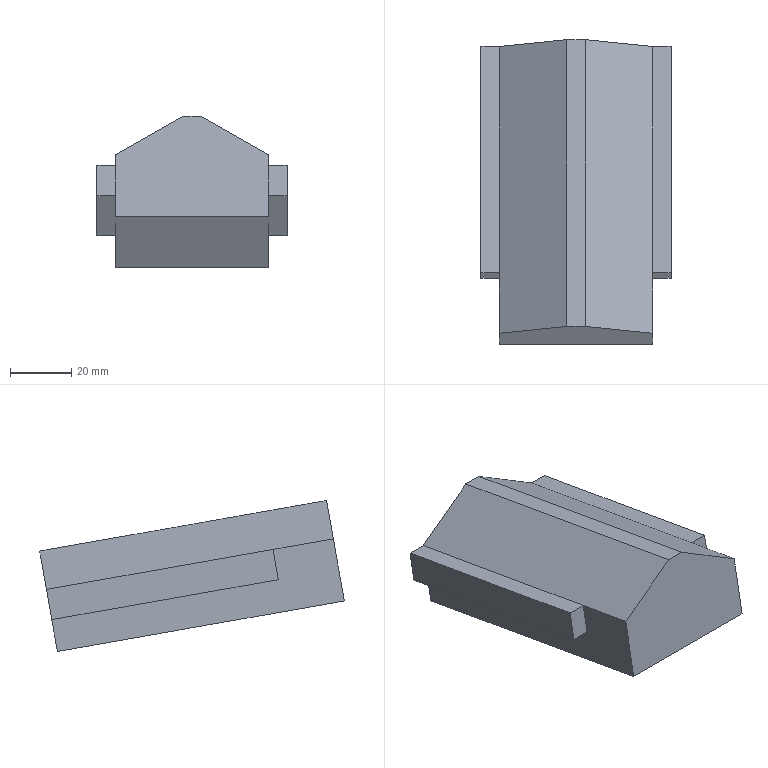Part | NX | features solid 2 | 1 solid | 16 faces | box 62 x 99.334 x 49.259 mm | volume 140476 mm3 | plane 16
STEP:
#1=CARTESIAN_POINT('',(-435.,-638.798,-53.975));
#2=VERTEX_POINT('',#1);
#3=CARTESIAN_POINT('',(-435.,-640.633,-64.38));
#4=VERTEX_POINT('',#3);
#5=CARTESIAN_POINT('',(-435.,-637.061,-44.126));
#6=DIRECTION('',(0.,-0.1736,-0.9848));
#7=VECTOR('',#6,1000.);
#8=LINE('',#5,#7);
#9=EDGE_CURVE('',#2,#4,#8,.T.);
#10=ORIENTED_EDGE('',*,*,#9,.T.);
#11=CARTESIAN_POINT('',(-435.,-734.189,-47.884));
#12=VERTEX_POINT('',#11);
#13=CARTESIAN_POINT('',(-435.,-734.189,-47.884));
#14=DIRECTION('',(0.,0.9848,-0.1736));
#15=VECTOR('',#14,1000.);
#16=LINE('',#13,#15);
#17=EDGE_CURVE('',#12,#4,#16,.T.);
#18=ORIENTED_EDGE('',*,*,#17,.F.);
#19=CARTESIAN_POINT('',(-435.,-732.354,-37.478));
#20=VERTEX_POINT('',#19);
#21=CARTESIAN_POINT('',(-435.,-730.618,-27.63));
#22=DIRECTION('',(0.,-0.1736,-0.9848));
#23=VECTOR('',#22,1000.);
#24=LINE('',#21,#23);
#25=EDGE_CURVE('',#20,#12,#24,.T.);
#26=ORIENTED_EDGE('',*,*,#25,.F.);
#27=CARTESIAN_POINT('',(-435.,-730.618,-27.63));
#28=VERTEX_POINT('',#27);
#29=CARTESIAN_POINT('',(-435.,-730.618,-27.63));
#30=CARTESIAN_POINT('',(-435.,-731.197,-30.913));
#31=CARTESIAN_POINT('',(-435.,-731.776,-34.195));
#32=CARTESIAN_POINT('',(-435.,-732.354,-37.478));
#33=B_SPLINE_CURVE_WITH_KNOTS('',3,(#29,#30,#31,#32),.UNSPECIFIED.,.F.,.F.,(4,4),(0.,1.),.PIECEWISE_BEZIER_KNOTS.);
#34=EDGE_CURVE('',#28,#20,#33,.T.);
#35=ORIENTED_EDGE('',*,*,#34,.F.);
#36=CARTESIAN_POINT('',(-435.,-710.922,-31.103));
#37=VERTEX_POINT('',#36);
#38=CARTESIAN_POINT('',(-435.,-710.922,-31.103));
#39=CARTESIAN_POINT('',(-435.,-717.487,-29.945));
#40=CARTESIAN_POINT('',(-435.,-724.053,-28.788));
#41=CARTESIAN_POINT('',(-435.,-730.618,-27.63));
#42=B_SPLINE_CURVE_WITH_KNOTS('',3,(#38,#39,#40,#41),.UNSPECIFIED.,.F.,.F.,(4,4),(0.,1.),.UNSPECIFIED.);
#43=EDGE_CURVE('',#28,#37,#42,.F.);
#44=ORIENTED_EDGE('',*,*,#43,.T.);
#45=CARTESIAN_POINT('',(-435.,-712.658,-40.951));
#46=VERTEX_POINT('',#45);
#47=CARTESIAN_POINT('',(-435.,-710.922,-31.103));
#48=CARTESIAN_POINT('',(-435.,-711.501,-34.386));
#49=CARTESIAN_POINT('',(-435.,-712.079,-37.668));
#50=CARTESIAN_POINT('',(-435.,-712.658,-40.951));
#51=B_SPLINE_CURVE_WITH_KNOTS('',3,(#47,#48,#49,#50),.UNSPECIFIED.,.F.,.F.,(4,4),(0.,1.),.PIECEWISE_BEZIER_KNOTS.);
#52=EDGE_CURVE('',#37,#46,#51,.T.);
#53=ORIENTED_EDGE('',*,*,#52,.T.);
#54=CARTESIAN_POINT('',(-435.,-673.266,-47.897));
#55=VERTEX_POINT('',#54);
#56=CARTESIAN_POINT('',(-435.,-732.354,-37.478));
#57=CARTESIAN_POINT('',(-435.,-712.658,-40.951));
#58=CARTESIAN_POINT('',(-435.,-692.962,-44.424));
#59=CARTESIAN_POINT('',(-435.,-673.266,-47.897));
#60=B_SPLINE_CURVE_WITH_KNOTS('',3,(#56,#57,#58,#59),.UNSPECIFIED.,.F.,.F.,(4,4),(0.,1.),.PIECEWISE_BEZIER_KNOTS.);
#61=EDGE_CURVE('',#55,#46,#60,.F.);
#62=ORIENTED_EDGE('',*,*,#61,.F.);
#63=CARTESIAN_POINT('',(-435.,-638.798,-53.975));
#64=DIRECTION('',(0.,-0.9848,0.1736));
#65=VECTOR('',#64,1000.);
#66=LINE('',#63,#65);
#67=EDGE_CURVE('',#2,#55,#66,.T.);
#68=ORIENTED_EDGE('',*,*,#67,.F.);
#69=EDGE_LOOP('',(#10,#18,#26,#35,#44,#53,#62,#68));
#70=FACE_BOUND('',#69,.T.);
#71=CARTESIAN_POINT('',(-435.,-730.618,-27.63));
#72=DIRECTION('',(-1.,0.,0.));
#73=DIRECTION('',(0.,0.342,-0.9397));
#74=AXIS2_PLACEMENT_3D('',#71,#72,#73);
#75=PLANE('',#74);
#76=ADVANCED_FACE('',(#70),#75,.T.);
#77=CARTESIAN_POINT('',(-385.,-730.618,-27.63));
#78=VERTEX_POINT('',#77);
#79=CARTESIAN_POINT('',(-385.,-732.354,-37.478));
#80=VERTEX_POINT('',#79);
#81=CARTESIAN_POINT('',(-385.,-730.618,-27.63));
#82=CARTESIAN_POINT('',(-385.,-731.197,-30.913));
#83=CARTESIAN_POINT('',(-385.,-731.776,-34.195));
#84=CARTESIAN_POINT('',(-385.,-732.354,-37.478));
#85=B_SPLINE_CURVE_WITH_KNOTS('',3,(#81,#82,#83,#84),.UNSPECIFIED.,.F.,.F.,(4,4),(0.,1.),.PIECEWISE_BEZIER_KNOTS.);
#86=EDGE_CURVE('',#78,#80,#85,.T.);
#87=ORIENTED_EDGE('',*,*,#86,.F.);
#88=CARTESIAN_POINT('',(-407.,-728.412,-15.121));
#89=VERTEX_POINT('',#88);
#90=CARTESIAN_POINT('',(-407.,-728.412,-15.121));
#91=DIRECTION('',(0.866,-0.08682,-0.4924));
#92=VECTOR('',#91,1000.);
#93=LINE('',#90,#92);
#94=EDGE_CURVE('',#89,#78,#93,.T.);
#95=ORIENTED_EDGE('',*,*,#94,.F.);
#96=CARTESIAN_POINT('',(-413.,-728.412,-15.121));
#97=VERTEX_POINT('',#96);
#98=CARTESIAN_POINT('',(-413.,-728.412,-15.121));
#99=DIRECTION('',(1.,0.,0.));
#100=VECTOR('',#99,1000.);
#101=LINE('',#98,#100);
#102=EDGE_CURVE('',#97,#89,#101,.T.);
#103=ORIENTED_EDGE('',*,*,#102,.F.);
#104=CARTESIAN_POINT('',(-435.,-730.618,-27.63));
#105=DIRECTION('',(0.866,0.08682,0.4924));
#106=VECTOR('',#105,1000.);
#107=LINE('',#104,#106);
#108=EDGE_CURVE('',#28,#97,#107,.T.);
#109=ORIENTED_EDGE('',*,*,#108,.F.);
#110=ORIENTED_EDGE('',*,*,#34,.T.);
#111=ORIENTED_EDGE('',*,*,#25,.T.);
#112=CARTESIAN_POINT('',(-385.,-734.189,-47.884));
#113=VERTEX_POINT('',#112);
#114=CARTESIAN_POINT('',(-435.,-734.189,-47.884));
#115=DIRECTION('',(1.,0.,0.));
#116=VECTOR('',#115,1000.);
#117=LINE('',#114,#116);
#118=EDGE_CURVE('',#12,#113,#117,.T.);
#119=ORIENTED_EDGE('',*,*,#118,.T.);
#120=CARTESIAN_POINT('',(-385.,-730.618,-27.63));
#121=DIRECTION('',(0.,-0.1736,-0.9848));
#122=VECTOR('',#121,1000.);
#123=LINE('',#120,#122);
#124=EDGE_CURVE('',#80,#113,#123,.T.);
#125=ORIENTED_EDGE('',*,*,#124,.F.);
#126=EDGE_LOOP('',(#87,#95,#103,#109,#110,#111,#119,#125));
#127=FACE_BOUND('',#126,.T.);
#128=CARTESIAN_POINT('',(-385.,-734.189,-47.884));
#129=DIRECTION('',(0.,-0.9848,0.1736));
#130=DIRECTION('',(0.,-0.1736,-0.9848));
#131=AXIS2_PLACEMENT_3D('',#128,#129,#130);
#132=PLANE('',#131);
#133=ADVANCED_FACE('',(#127),#132,.T.);
#134=CARTESIAN_POINT('',(-385.,-640.633,-64.38));
#135=VERTEX_POINT('',#134);
#136=CARTESIAN_POINT('',(-435.,-640.633,-64.38));
#137=DIRECTION('',(1.,0.,0.));
#138=VECTOR('',#137,1000.);
#139=LINE('',#136,#138);
#140=EDGE_CURVE('',#4,#135,#139,.T.);
#141=ORIENTED_EDGE('',*,*,#140,.T.);
#142=CARTESIAN_POINT('',(-385.,-734.189,-47.884));
#143=DIRECTION('',(0.,0.9848,-0.1736));
#144=VECTOR('',#143,1000.);
#145=LINE('',#142,#144);
#146=EDGE_CURVE('',#113,#135,#145,.T.);
#147=ORIENTED_EDGE('',*,*,#146,.F.);
#148=ORIENTED_EDGE('',*,*,#118,.F.);
#149=ORIENTED_EDGE('',*,*,#17,.T.);
#150=EDGE_LOOP('',(#141,#147,#148,#149));
#151=FACE_BOUND('',#150,.T.);
#152=CARTESIAN_POINT('',(-435.,-734.189,-47.884));
#153=DIRECTION('',(0.,-0.1736,-0.9848));
#154=DIRECTION('',(0.,0.9848,-0.1736));
#155=AXIS2_PLACEMENT_3D('',#152,#153,#154);
#156=PLANE('',#155);
#157=ADVANCED_FACE('',(#151),#156,.T.);
#158=CARTESIAN_POINT('',(-385.,-712.658,-40.951));
#159=VERTEX_POINT('',#158);
#160=CARTESIAN_POINT('',(-385.,-673.266,-47.897));
#161=VERTEX_POINT('',#160);
#162=CARTESIAN_POINT('',(-385.,-732.354,-37.478));
#163=CARTESIAN_POINT('',(-385.,-712.658,-40.951));
#164=CARTESIAN_POINT('',(-385.,-692.962,-44.424));
#165=CARTESIAN_POINT('',(-385.,-673.266,-47.897));
#166=B_SPLINE_CURVE_WITH_KNOTS('',3,(#162,#163,#164,#165),.UNSPECIFIED.,.F.,.F.,(4,4),(0.,1.),.PIECEWISE_BEZIER_KNOTS.);
#167=EDGE_CURVE('',#159,#161,#166,.T.);
#168=ORIENTED_EDGE('',*,*,#167,.F.);
#169=CARTESIAN_POINT('',(-385.,-710.922,-31.103));
#170=VERTEX_POINT('',#169);
#171=CARTESIAN_POINT('',(-385.,-710.922,-31.103));
#172=CARTESIAN_POINT('',(-385.,-711.501,-34.386));
#173=CARTESIAN_POINT('',(-385.,-712.079,-37.668));
#174=CARTESIAN_POINT('',(-385.,-712.658,-40.951));
#175=B_SPLINE_CURVE_WITH_KNOTS('',3,(#171,#172,#173,#174),.UNSPECIFIED.,.F.,.F.,(4,4),(0.,1.),.PIECEWISE_BEZIER_KNOTS.);
#176=EDGE_CURVE('',#170,#159,#175,.T.);
#177=ORIENTED_EDGE('',*,*,#176,.F.);
#178=CARTESIAN_POINT('',(-385.,-730.618,-27.63));
#179=CARTESIAN_POINT('',(-385.,-724.053,-28.788));
#180=CARTESIAN_POINT('',(-385.,-717.487,-29.945));
#181=CARTESIAN_POINT('',(-385.,-710.922,-31.103));
#182=B_SPLINE_CURVE_WITH_KNOTS('',3,(#178,#179,#180,#181),.UNSPECIFIED.,.F.,.F.,(4,4),(0.,1.),.UNSPECIFIED.);
#183=EDGE_CURVE('',#78,#170,#182,.T.);
#184=ORIENTED_EDGE('',*,*,#183,.F.);
#185=ORIENTED_EDGE('',*,*,#86,.T.);
#186=ORIENTED_EDGE('',*,*,#124,.T.);
#187=ORIENTED_EDGE('',*,*,#146,.T.);
#188=CARTESIAN_POINT('',(-385.,-638.798,-53.975));
#189=VERTEX_POINT('',#188);
#190=CARTESIAN_POINT('',(-385.,-637.061,-44.126));
#191=DIRECTION('',(0.,-0.1736,-0.9848));
#192=VECTOR('',#191,1000.);
#193=LINE('',#190,#192);
#194=EDGE_CURVE('',#189,#135,#193,.T.);
#195=ORIENTED_EDGE('',*,*,#194,.F.);
#196=CARTESIAN_POINT('',(-385.,-638.798,-53.975));
#197=DIRECTION('',(0.,-0.9848,0.1736));
#198=VECTOR('',#197,1000.);
#199=LINE('',#196,#198);
#200=EDGE_CURVE('',#161,#189,#199,.F.);
#201=ORIENTED_EDGE('',*,*,#200,.F.);
#202=EDGE_LOOP('',(#168,#177,#184,#185,#186,#187,#195,#201));
#203=FACE_BOUND('',#202,.T.);
#204=CARTESIAN_POINT('',(-385.,-730.618,-27.63));
#205=DIRECTION('',(-1.,0.,0.));
#206=DIRECTION('',(0.,0.9397,0.342));
#207=AXIS2_PLACEMENT_3D('',#204,#205,#206);
#208=PLANE('',#207);
#209=ADVANCED_FACE('',(#203),#208,.F.);
#210=CARTESIAN_POINT('',(-407.,-634.856,-31.618));
#211=VERTEX_POINT('',#210);
#212=CARTESIAN_POINT('',(-385.,-637.061,-44.126));
#213=VERTEX_POINT('',#212);
#214=CARTESIAN_POINT('',(-407.,-634.856,-31.618));
#215=DIRECTION('',(0.866,-0.08682,-0.4924));
#216=VECTOR('',#215,1000.);
#217=LINE('',#214,#216);
#218=EDGE_CURVE('',#211,#213,#217,.T.);
#219=ORIENTED_EDGE('',*,*,#218,.F.);
#220=CARTESIAN_POINT('',(-407.,-728.412,-15.121));
#221=DIRECTION('',(0.,0.9848,-0.1736));
#222=VECTOR('',#221,1000.);
#223=LINE('',#220,#222);
#224=EDGE_CURVE('',#89,#211,#223,.T.);
#225=ORIENTED_EDGE('',*,*,#224,.F.);
#226=ORIENTED_EDGE('',*,*,#94,.T.);
#227=ORIENTED_EDGE('',*,*,#183,.T.);
#228=CARTESIAN_POINT('',(-385.,-671.53,-38.049));
#229=VERTEX_POINT('',#228);
#230=CARTESIAN_POINT('',(-385.,-730.618,-27.63));
#231=DIRECTION('',(0.,0.9848,-0.1736));
#232=VECTOR('',#231,1000.);
#233=LINE('',#230,#232);
#234=EDGE_CURVE('',#170,#229,#233,.T.);
#235=ORIENTED_EDGE('',*,*,#234,.T.);
#236=CARTESIAN_POINT('',(-385.,-637.061,-44.126));
#237=CARTESIAN_POINT('',(-385.,-648.551,-42.101));
#238=CARTESIAN_POINT('',(-385.,-660.04,-40.075));
#239=CARTESIAN_POINT('',(-385.,-671.53,-38.049));
#240=B_SPLINE_CURVE_WITH_KNOTS('',3,(#236,#237,#238,#239),.UNSPECIFIED.,.F.,.F.,(4,4),(0.,1.),.UNSPECIFIED.);
#241=EDGE_CURVE('',#229,#213,#240,.F.);
#242=ORIENTED_EDGE('',*,*,#241,.T.);
#243=EDGE_LOOP('',(#219,#225,#226,#227,#235,#242));
#244=FACE_BOUND('',#243,.T.);
#245=CARTESIAN_POINT('',(-407.,-728.412,-15.121));
#246=DIRECTION('',(-0.5,-0.1504,-0.8529));
#247=DIRECTION('',(0.8321,0.1897,-0.5212));
#248=AXIS2_PLACEMENT_3D('',#245,#246,#247);
#249=PLANE('',#248);
#250=ADVANCED_FACE('',(#244),#249,.F.);
#251=CARTESIAN_POINT('',(-413.,-634.856,-31.618));
#252=VERTEX_POINT('',#251);
#253=CARTESIAN_POINT('',(-413.,-634.856,-31.618));
#254=DIRECTION('',(1.,0.,0.));
#255=VECTOR('',#254,1000.);
#256=LINE('',#253,#255);
#257=EDGE_CURVE('',#252,#211,#256,.T.);
#258=ORIENTED_EDGE('',*,*,#257,.F.);
#259=CARTESIAN_POINT('',(-413.,-728.412,-15.121));
#260=DIRECTION('',(0.,0.9848,-0.1736));
#261=VECTOR('',#260,1000.);
#262=LINE('',#259,#261);
#263=EDGE_CURVE('',#97,#252,#262,.T.);
#264=ORIENTED_EDGE('',*,*,#263,.F.);
#265=ORIENTED_EDGE('',*,*,#102,.T.);
#266=ORIENTED_EDGE('',*,*,#224,.T.);
#267=EDGE_LOOP('',(#258,#264,#265,#266));
#268=FACE_BOUND('',#267,.T.);
#269=CARTESIAN_POINT('',(-413.,-728.412,-15.121));
#270=DIRECTION('',(0.,-0.1736,-0.9848));
#271=DIRECTION('',(0.,0.9848,-0.1736));
#272=AXIS2_PLACEMENT_3D('',#269,#270,#271);
#273=PLANE('',#272);
#274=ADVANCED_FACE('',(#268),#273,.F.);
#275=CARTESIAN_POINT('',(-435.,-637.061,-44.126));
#276=VERTEX_POINT('',#275);
#277=CARTESIAN_POINT('',(-435.,-637.061,-44.126));
#278=DIRECTION('',(0.866,0.08682,0.4924));
#279=VECTOR('',#278,1000.);
#280=LINE('',#277,#279);
#281=EDGE_CURVE('',#276,#252,#280,.T.);
#282=ORIENTED_EDGE('',*,*,#281,.F.);
#283=CARTESIAN_POINT('',(-435.,-671.53,-38.049));
#284=VERTEX_POINT('',#283);
#285=CARTESIAN_POINT('',(-435.,-671.53,-38.049));
#286=CARTESIAN_POINT('',(-435.,-660.04,-40.075));
#287=CARTESIAN_POINT('',(-435.,-648.551,-42.101));
#288=CARTESIAN_POINT('',(-435.,-637.061,-44.126));
#289=B_SPLINE_CURVE_WITH_KNOTS('',3,(#285,#286,#287,#288),.UNSPECIFIED.,.F.,.F.,(4,4),(0.,1.),.UNSPECIFIED.);
#290=EDGE_CURVE('',#284,#276,#289,.T.);
#291=ORIENTED_EDGE('',*,*,#290,.F.);
#292=CARTESIAN_POINT('',(-435.,-730.618,-27.63));
#293=DIRECTION('',(0.,0.9848,-0.1736));
#294=VECTOR('',#293,1000.);
#295=LINE('',#292,#294);
#296=EDGE_CURVE('',#37,#284,#295,.T.);
#297=ORIENTED_EDGE('',*,*,#296,.F.);
#298=ORIENTED_EDGE('',*,*,#43,.F.);
#299=ORIENTED_EDGE('',*,*,#108,.T.);
#300=ORIENTED_EDGE('',*,*,#263,.T.);
#301=EDGE_LOOP('',(#282,#291,#297,#298,#299,#300));
#302=FACE_BOUND('',#301,.T.);
#303=CARTESIAN_POINT('',(-435.,-730.618,-27.63));
#304=DIRECTION('',(0.5,-0.1504,-0.8529));
#305=DIRECTION('',(0.8321,-0.1897,0.5212));
#306=AXIS2_PLACEMENT_3D('',#303,#304,#305);
#307=PLANE('',#306);
#308=ADVANCED_FACE('',(#302),#307,.F.);
#309=ORIENTED_EDGE('',*,*,#140,.F.);
#310=ORIENTED_EDGE('',*,*,#9,.F.);
#311=CARTESIAN_POINT('',(-441.,-638.798,-53.975));
#312=VERTEX_POINT('',#311);
#313=CARTESIAN_POINT('',(-441.,-638.798,-53.975));
#314=DIRECTION('',(1.,0.,0.));
#315=VECTOR('',#314,1000.);
#316=LINE('',#313,#315);
#317=EDGE_CURVE('',#312,#2,#316,.T.);
#318=ORIENTED_EDGE('',*,*,#317,.F.);
#319=CARTESIAN_POINT('',(-441.,-637.061,-44.126));
#320=VERTEX_POINT('',#319);
#321=CARTESIAN_POINT('',(-441.,-637.061,-44.126));
#322=CARTESIAN_POINT('',(-441.,-637.64,-47.409));
#323=CARTESIAN_POINT('',(-441.,-638.219,-50.692));
#324=CARTESIAN_POINT('',(-441.,-638.798,-53.975));
#325=B_SPLINE_CURVE_WITH_KNOTS('',3,(#321,#322,#323,#324),.UNSPECIFIED.,.F.,.F.,(4,4),(0.,1.),.PIECEWISE_BEZIER_KNOTS.);
#326=EDGE_CURVE('',#320,#312,#325,.T.);
#327=ORIENTED_EDGE('',*,*,#326,.F.);
#328=CARTESIAN_POINT('',(-441.,-637.061,-44.126));
#329=DIRECTION('',(1.,0.,0.));
#330=VECTOR('',#329,1000.);
#331=LINE('',#328,#330);
#332=EDGE_CURVE('',#320,#276,#331,.T.);
#333=ORIENTED_EDGE('',*,*,#332,.T.);
#334=ORIENTED_EDGE('',*,*,#281,.T.);
#335=ORIENTED_EDGE('',*,*,#257,.T.);
#336=ORIENTED_EDGE('',*,*,#218,.T.);
#337=CARTESIAN_POINT('',(-379.,-637.061,-44.126));
#338=VERTEX_POINT('',#337);
#339=CARTESIAN_POINT('',(-379.,-637.061,-44.126));
#340=DIRECTION('',(-1.,0.,0.));
#341=VECTOR('',#340,1000.);
#342=LINE('',#339,#341);
#343=EDGE_CURVE('',#338,#213,#342,.T.);
#344=ORIENTED_EDGE('',*,*,#343,.F.);
#345=CARTESIAN_POINT('',(-379.,-638.798,-53.975));
#346=VERTEX_POINT('',#345);
#347=CARTESIAN_POINT('',(-379.,-637.061,-44.126));
#348=CARTESIAN_POINT('',(-379.,-637.64,-47.409));
#349=CARTESIAN_POINT('',(-379.,-638.219,-50.692));
#350=CARTESIAN_POINT('',(-379.,-638.798,-53.975));
#351=B_SPLINE_CURVE_WITH_KNOTS('',3,(#347,#348,#349,#350),.UNSPECIFIED.,.F.,.F.,(4,4),(0.,1.),.PIECEWISE_BEZIER_KNOTS.);
#352=EDGE_CURVE('',#338,#346,#351,.T.);
#353=ORIENTED_EDGE('',*,*,#352,.T.);
#354=CARTESIAN_POINT('',(-379.,-638.798,-53.975));
#355=DIRECTION('',(-1.,0.,0.));
#356=VECTOR('',#355,1000.);
#357=LINE('',#354,#356);
#358=EDGE_CURVE('',#346,#189,#357,.T.);
#359=ORIENTED_EDGE('',*,*,#358,.T.);
#360=ORIENTED_EDGE('',*,*,#194,.T.);
#361=EDGE_LOOP('',(#309,#310,#318,#327,#333,#334,#335,#336,#344,#353,#359,#360));
#362=FACE_BOUND('',#361,.T.);
#363=CARTESIAN_POINT('',(-385.,-640.633,-64.38));
#364=DIRECTION('',(0.,-0.9848,0.1736));
#365=DIRECTION('',(0.,-0.1736,-0.9848));
#366=AXIS2_PLACEMENT_3D('',#363,#364,#365);
#367=PLANE('',#366);
#368=ADVANCED_FACE('',(#362),#367,.F.);
#369=CARTESIAN_POINT('',(-441.,-710.922,-31.103));
#370=VERTEX_POINT('',#369);
#371=CARTESIAN_POINT('',(-441.,-710.922,-31.103));
#372=DIRECTION('',(1.,0.,0.));
#373=VECTOR('',#372,1000.);
#374=LINE('',#371,#373);
#375=EDGE_CURVE('',#370,#37,#374,.T.);
#376=ORIENTED_EDGE('',*,*,#375,.T.);
#377=ORIENTED_EDGE('',*,*,#296,.T.);
#378=ORIENTED_EDGE('',*,*,#290,.T.);
#379=ORIENTED_EDGE('',*,*,#332,.F.);
#380=CARTESIAN_POINT('',(-441.,-671.53,-38.049));
#381=VERTEX_POINT('',#380);
#382=CARTESIAN_POINT('',(-441.,-637.061,-44.126));
#383=DIRECTION('',(0.,-0.9848,0.1736));
#384=VECTOR('',#383,1000.);
#385=LINE('',#382,#384);
#386=EDGE_CURVE('',#381,#320,#385,.F.);
#387=ORIENTED_EDGE('',*,*,#386,.F.);
#388=CARTESIAN_POINT('',(-441.,-730.618,-27.63));
#389=DIRECTION('',(0.,0.9848,-0.1736));
#390=VECTOR('',#389,1000.);
#391=LINE('',#388,#390);
#392=EDGE_CURVE('',#370,#381,#391,.T.);
#393=ORIENTED_EDGE('',*,*,#392,.F.);
#394=EDGE_LOOP('',(#376,#377,#378,#379,#387,#393));
#395=FACE_BOUND('',#394,.T.);
#396=CARTESIAN_POINT('',(-441.,-730.618,-27.63));
#397=DIRECTION('',(0.,0.1736,0.9848));
#398=DIRECTION('',(0.,-0.9848,0.1736));
#399=AXIS2_PLACEMENT_3D('',#396,#397,#398);
#400=PLANE('',#399);
#401=ADVANCED_FACE('',(#395),#400,.T.);
#402=CARTESIAN_POINT('',(-441.,-712.658,-40.951));
#403=VERTEX_POINT('',#402);
#404=CARTESIAN_POINT('',(-441.,-673.266,-47.897));
#405=VERTEX_POINT('',#404);
#406=CARTESIAN_POINT('',(-441.,-732.354,-37.478));
#407=CARTESIAN_POINT('',(-441.,-712.658,-40.951));
#408=CARTESIAN_POINT('',(-441.,-692.962,-44.424));
#409=CARTESIAN_POINT('',(-441.,-673.266,-47.897));
#410=B_SPLINE_CURVE_WITH_KNOTS('',3,(#406,#407,#408,#409),.UNSPECIFIED.,.F.,.F.,(4,4),(0.,1.),.PIECEWISE_BEZIER_KNOTS.);
#411=EDGE_CURVE('',#403,#405,#410,.T.);
#412=ORIENTED_EDGE('',*,*,#411,.T.);
#413=CARTESIAN_POINT('',(-441.,-638.798,-53.975));
#414=DIRECTION('',(0.,-0.9848,0.1736));
#415=VECTOR('',#414,1000.);
#416=LINE('',#413,#415);
#417=EDGE_CURVE('',#405,#312,#416,.F.);
#418=ORIENTED_EDGE('',*,*,#417,.T.);
#419=ORIENTED_EDGE('',*,*,#317,.T.);
#420=ORIENTED_EDGE('',*,*,#67,.T.);
#421=ORIENTED_EDGE('',*,*,#61,.T.);
#422=CARTESIAN_POINT('',(-441.,-712.658,-40.951));
#423=DIRECTION('',(1.,0.,0.));
#424=VECTOR('',#423,1000.);
#425=LINE('',#422,#424);
#426=EDGE_CURVE('',#403,#46,#425,.T.);
#427=ORIENTED_EDGE('',*,*,#426,.F.);
#428=EDGE_LOOP('',(#412,#418,#419,#420,#421,#427));
#429=FACE_BOUND('',#428,.T.);
#430=CARTESIAN_POINT('',(-441.,-732.354,-37.478));
#431=DIRECTION('',(0.,0.1736,0.9848));
#432=DIRECTION('',(0.,-0.9848,0.1736));
#433=AXIS2_PLACEMENT_3D('',#430,#431,#432);
#434=PLANE('',#433);
#435=ADVANCED_FACE('',(#429),#434,.F.);
#436=CARTESIAN_POINT('',(-441.,-710.922,-31.103));
#437=CARTESIAN_POINT('',(-441.,-711.501,-34.386));
#438=CARTESIAN_POINT('',(-441.,-712.079,-37.668));
#439=CARTESIAN_POINT('',(-441.,-712.658,-40.951));
#440=B_SPLINE_CURVE_WITH_KNOTS('',3,(#436,#437,#438,#439),.UNSPECIFIED.,.F.,.F.,(4,4),(0.,1.),.PIECEWISE_BEZIER_KNOTS.);
#441=EDGE_CURVE('',#370,#403,#440,.T.);
#442=ORIENTED_EDGE('',*,*,#441,.F.);
#443=ORIENTED_EDGE('',*,*,#392,.T.);
#444=ORIENTED_EDGE('',*,*,#386,.T.);
#445=ORIENTED_EDGE('',*,*,#326,.T.);
#446=ORIENTED_EDGE('',*,*,#417,.F.);
#447=ORIENTED_EDGE('',*,*,#411,.F.);
#448=EDGE_LOOP('',(#442,#443,#444,#445,#446,#447));
#449=FACE_BOUND('',#448,.T.);
#450=CARTESIAN_POINT('',(-441.,-732.354,-37.478));
#451=DIRECTION('',(-1.,0.,0.));
#452=DIRECTION('',(0.,0.342,-0.9397));
#453=AXIS2_PLACEMENT_3D('',#450,#451,#452);
#454=PLANE('',#453);
#455=ADVANCED_FACE('',(#449),#454,.T.);
#456=CARTESIAN_POINT('',(-379.,-710.922,-31.103));
#457=VERTEX_POINT('',#456);
#458=CARTESIAN_POINT('',(-379.,-710.922,-31.103));
#459=DIRECTION('',(-1.,0.,0.));
#460=VECTOR('',#459,1000.);
#461=LINE('',#458,#460);
#462=EDGE_CURVE('',#457,#170,#461,.T.);
#463=ORIENTED_EDGE('',*,*,#462,.F.);
#464=CARTESIAN_POINT('',(-379.,-671.53,-38.049));
#465=VERTEX_POINT('',#464);
#466=CARTESIAN_POINT('',(-379.,-730.618,-27.63));
#467=DIRECTION('',(0.,0.9848,-0.1736));
#468=VECTOR('',#467,1000.);
#469=LINE('',#466,#468);
#470=EDGE_CURVE('',#457,#465,#469,.T.);
#471=ORIENTED_EDGE('',*,*,#470,.T.);
#472=CARTESIAN_POINT('',(-379.,-637.061,-44.126));
#473=DIRECTION('',(0.,-0.9848,0.1736));
#474=VECTOR('',#473,1000.);
#475=LINE('',#472,#474);
#476=EDGE_CURVE('',#465,#338,#475,.F.);
#477=ORIENTED_EDGE('',*,*,#476,.T.);
#478=ORIENTED_EDGE('',*,*,#343,.T.);
#479=ORIENTED_EDGE('',*,*,#241,.F.);
#480=ORIENTED_EDGE('',*,*,#234,.F.);
#481=EDGE_LOOP('',(#463,#471,#477,#478,#479,#480));
#482=FACE_BOUND('',#481,.T.);
#483=CARTESIAN_POINT('',(-379.,-730.618,-27.63));
#484=DIRECTION('',(0.,0.1736,0.9848));
#485=DIRECTION('',(0.,-0.9848,0.1736));
#486=AXIS2_PLACEMENT_3D('',#483,#484,#485);
#487=PLANE('',#486);
#488=ADVANCED_FACE('',(#482),#487,.T.);
#489=ORIENTED_EDGE('',*,*,#167,.T.);
#490=ORIENTED_EDGE('',*,*,#200,.T.);
#491=ORIENTED_EDGE('',*,*,#358,.F.);
#492=CARTESIAN_POINT('',(-379.,-673.266,-47.897));
#493=VERTEX_POINT('',#492);
#494=CARTESIAN_POINT('',(-379.,-638.798,-53.975));
#495=DIRECTION('',(0.,-0.9848,0.1736));
#496=VECTOR('',#495,1000.);
#497=LINE('',#494,#496);
#498=EDGE_CURVE('',#493,#346,#497,.F.);
#499=ORIENTED_EDGE('',*,*,#498,.F.);
#500=CARTESIAN_POINT('',(-379.,-712.658,-40.951));
#501=VERTEX_POINT('',#500);
#502=CARTESIAN_POINT('',(-379.,-732.354,-37.478));
#503=CARTESIAN_POINT('',(-379.,-712.658,-40.951));
#504=CARTESIAN_POINT('',(-379.,-692.962,-44.424));
#505=CARTESIAN_POINT('',(-379.,-673.266,-47.897));
#506=B_SPLINE_CURVE_WITH_KNOTS('',3,(#502,#503,#504,#505),.UNSPECIFIED.,.F.,.F.,(4,4),(0.,1.),.PIECEWISE_BEZIER_KNOTS.);
#507=EDGE_CURVE('',#501,#493,#506,.T.);
#508=ORIENTED_EDGE('',*,*,#507,.F.);
#509=CARTESIAN_POINT('',(-379.,-712.658,-40.951));
#510=DIRECTION('',(-1.,0.,0.));
#511=VECTOR('',#510,1000.);
#512=LINE('',#509,#511);
#513=EDGE_CURVE('',#501,#159,#512,.T.);
#514=ORIENTED_EDGE('',*,*,#513,.T.);
#515=EDGE_LOOP('',(#489,#490,#491,#499,#508,#514));
#516=FACE_BOUND('',#515,.T.);
#517=CARTESIAN_POINT('',(-379.,-732.354,-37.478));
#518=DIRECTION('',(0.,0.1736,0.9848));
#519=DIRECTION('',(0.,-0.9848,0.1736));
#520=AXIS2_PLACEMENT_3D('',#517,#518,#519);
#521=PLANE('',#520);
#522=ADVANCED_FACE('',(#516),#521,.F.);
#523=CARTESIAN_POINT('',(-379.,-710.922,-31.103));
#524=CARTESIAN_POINT('',(-379.,-711.501,-34.386));
#525=CARTESIAN_POINT('',(-379.,-712.079,-37.668));
#526=CARTESIAN_POINT('',(-379.,-712.658,-40.951));
#527=B_SPLINE_CURVE_WITH_KNOTS('',3,(#523,#524,#525,#526),.UNSPECIFIED.,.F.,.F.,(4,4),(0.,1.),.PIECEWISE_BEZIER_KNOTS.);
#528=EDGE_CURVE('',#457,#501,#527,.T.);
#529=ORIENTED_EDGE('',*,*,#528,.T.);
#530=ORIENTED_EDGE('',*,*,#507,.T.);
#531=ORIENTED_EDGE('',*,*,#498,.T.);
#532=ORIENTED_EDGE('',*,*,#352,.F.);
#533=ORIENTED_EDGE('',*,*,#476,.F.);
#534=ORIENTED_EDGE('',*,*,#470,.F.);
#535=EDGE_LOOP('',(#529,#530,#531,#532,#533,#534));
#536=FACE_BOUND('',#535,.T.);
#537=CARTESIAN_POINT('',(-379.,-732.354,-37.478));
#538=DIRECTION('',(1.,0.,0.));
#539=DIRECTION('',(0.,0.342,-0.9397));
#540=AXIS2_PLACEMENT_3D('',#537,#538,#539);
#541=PLANE('',#540);
#542=ADVANCED_FACE('',(#536),#541,.T.);
#543=ORIENTED_EDGE('',*,*,#52,.F.);
#544=ORIENTED_EDGE('',*,*,#375,.F.);
#545=ORIENTED_EDGE('',*,*,#441,.T.);
#546=ORIENTED_EDGE('',*,*,#426,.T.);
#547=EDGE_LOOP('',(#543,#544,#545,#546));
#548=FACE_BOUND('',#547,.T.);
#549=CARTESIAN_POINT('',(-441.,-710.922,-31.103));
#550=DIRECTION('',(0.,0.9848,-0.1736));
#551=DIRECTION('',(0.,0.1736,0.9848));
#552=AXIS2_PLACEMENT_3D('',#549,#550,#551);
#553=PLANE('',#552);
#554=ADVANCED_FACE('',(#548),#553,.F.);
#555=ORIENTED_EDGE('',*,*,#176,.T.);
#556=ORIENTED_EDGE('',*,*,#513,.F.);
#557=ORIENTED_EDGE('',*,*,#528,.F.);
#558=ORIENTED_EDGE('',*,*,#462,.T.);
#559=EDGE_LOOP('',(#555,#556,#557,#558));
#560=FACE_BOUND('',#559,.T.);
#561=CARTESIAN_POINT('',(-379.,-710.922,-31.103));
#562=DIRECTION('',(0.,0.9848,-0.1736));
#563=DIRECTION('',(0.,0.1736,0.9848));
#564=AXIS2_PLACEMENT_3D('',#561,#562,#563);
#565=PLANE('',#564);
#566=ADVANCED_FACE('',(#560),#565,.F.);
#567=CLOSED_SHELL('',(#76,#133,#157,#209,#250,#274,#308,#368,#401,#435,#455,#488,#522,#542,#554,#566));
#568=MANIFOLD_SOLID_BREP('',#567);
#569=(LENGTH_UNIT()NAMED_UNIT(*)SI_UNIT(.MILLI.,.METRE.));
#570=UNCERTAINTY_MEASURE_WITH_UNIT(LENGTH_MEASURE(0.0508),#569,'','');
#571=(NAMED_UNIT(*)PLANE_ANGLE_UNIT()SI_UNIT($,.RADIAN.));
#572=(NAMED_UNIT(*)SI_UNIT($,.STERADIAN.)SOLID_ANGLE_UNIT());
#573=(GEOMETRIC_REPRESENTATION_CONTEXT(3)GLOBAL_UNCERTAINTY_ASSIGNED_CONTEXT((#570))GLOBAL_UNIT_ASSIGNED_CONTEXT((#569,#571,#572))REPRESENTATION_CONTEXT('',''));
#574=ADVANCED_BREP_SHAPE_REPRESENTATION('',(#568),#573);